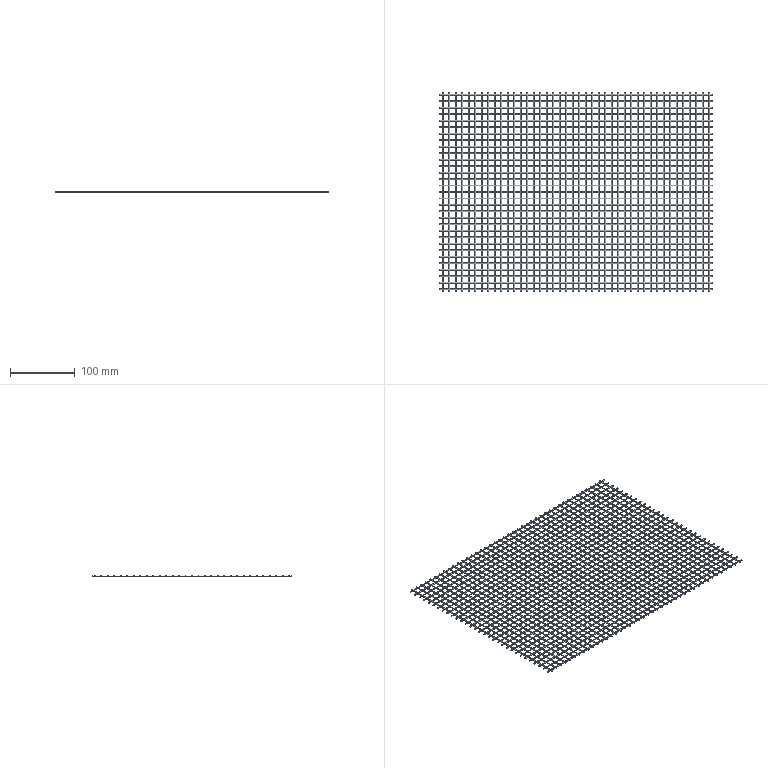Part | STEP file | 750078418 | 73 solids | 292 faces | box 422 x 305.5 x 1.5 mm | volume 45792 mm3 | cylinder 146 | plane 146 | commonest cylinder face diameters 1.5 x146